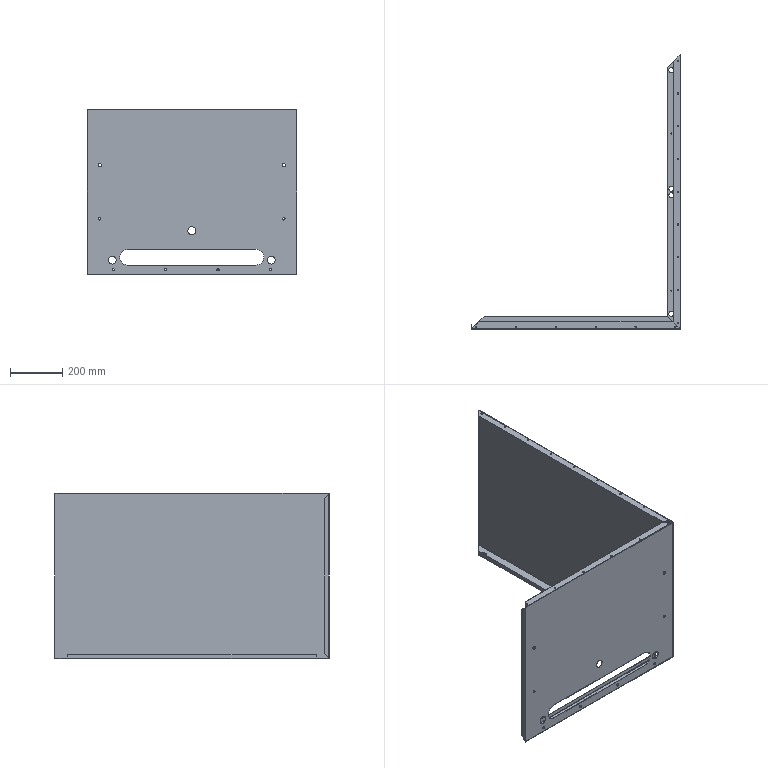Part | STEP file | HESS-408-70-15W-W-2-outer case side panel 2 | 1 solid | 146 faces | box 798.5 x 1049 x 630 mm | volume 1938320 mm3 | cylinder 82 | plane 58 | spline 6 | commonest cylinder face diameters 5 x30 9 x12 0.2 x8 3.2 x8 20 x8 30 x6